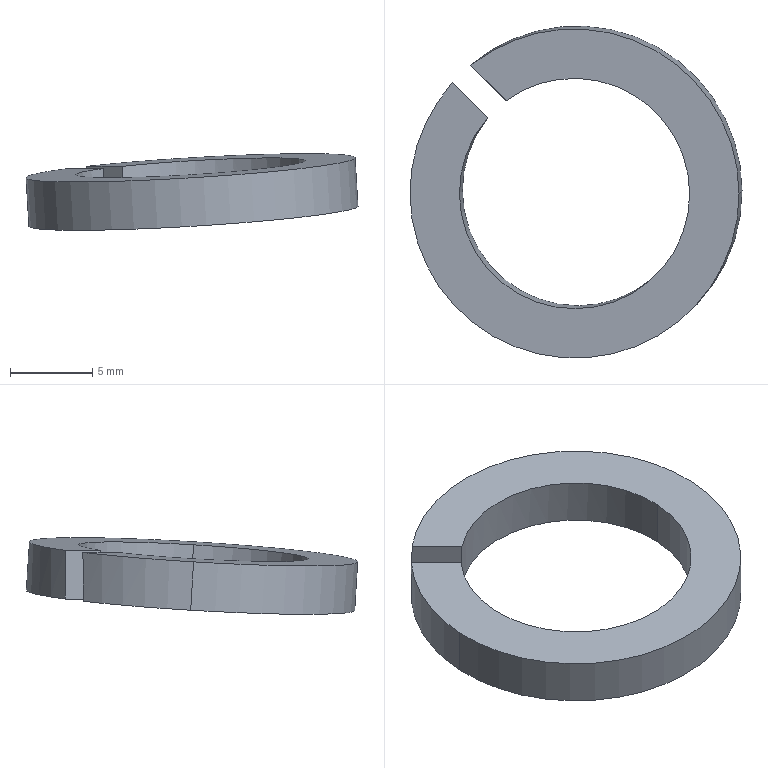Part | SolidWorks | features Boss 1, Cut 1, Extrusion 1, Helix 1, Sweep 1 | 1 solid | 10 faces | box 20.15 x 20.15 x 4.655 mm | volume 458.797 mm3 | cylinder 6 | plane 4 | commonest cylinder face diameters 14 x3 20.008 x3
STEP:
#1=CARTESIAN_POINT('',(-7.602,6.506,0.2121));
#2=VERTEX_POINT('',#1);
#3=CARTESIAN_POINT('',(-10.002,-0.01691,-0.3327));
#4=VERTEX_POINT('',#3);
#5=CARTESIAN_POINT('',(-0.01691,-0.01691,0.2769));
#6=DIRECTION('',(-0.06083,-0.06083,0.9963));
#7=DIRECTION('',(0.9981,0.,0.06094));
#8=AXIS2_PLACEMENT_3D('',#5,#6,#7);
#9=CIRCLE('',#8,10.004);
#10=EDGE_CURVE('',#2,#4,#9,.T.);
#11=ORIENTED_EDGE('',*,*,#10,.T.);
#12=CARTESIAN_POINT('',(-10.181,-0.196,2.601));
#13=VERTEX_POINT('',#12);
#14=CARTESIAN_POINT('',(-10.002,-0.01691,-0.3327));
#15=DIRECTION('',(-0.06083,-0.06083,0.9963));
#16=VECTOR('',#15,1000.);
#17=LINE('',#14,#16);
#18=EDGE_CURVE('',#4,#13,#17,.T.);
#19=ORIENTED_EDGE('',*,*,#18,.T.);
#20=CARTESIAN_POINT('',(-7.613,6.517,3.168));
#21=VERTEX_POINT('',#20);
#22=CARTESIAN_POINT('',(-0.196,-0.196,3.211));
#23=DIRECTION('',(-0.06083,-0.06083,0.9963));
#24=DIRECTION('',(0.9981,0.,0.06094));
#25=AXIS2_PLACEMENT_3D('',#22,#23,#24);
#26=CIRCLE('',#25,10.004);
#27=EDGE_CURVE('',#21,#13,#26,.T.);
#28=ORIENTED_EDGE('',*,*,#27,.F.);
#29=CARTESIAN_POINT('',(-7.602,6.506,0.2121));
#30=CARTESIAN_POINT('',(-7.606,6.51,1.197));
#31=CARTESIAN_POINT('',(-7.61,6.514,2.182));
#32=CARTESIAN_POINT('',(-7.613,6.517,3.168));
#33=(BOUNDED_CURVE()B_SPLINE_CURVE(3,(#29,#30,#31,#32),.UNSPECIFIED.,.F.,.F.)B_SPLINE_CURVE_WITH_KNOTS((4,4),(4.637,4.662),.UNSPECIFIED.)CURVE()GEOMETRIC_REPRESENTATION_ITEM()RATIONAL_B_SPLINE_CURVE((1.,0.9999,0.9999,1.))REPRESENTATION_ITEM(''));
#34=EDGE_CURVE('',#2,#21,#33,.T.);
#35=ORIENTED_EDGE('',*,*,#34,.F.);
#36=EDGE_LOOP('',(#11,#19,#28,#35));
#37=FACE_OUTER_BOUND('',#36,.T.);
#38=CARTESIAN_POINT('',(-0.01691,-0.01691,0.2769));
#39=DIRECTION('',(-0.06083,-0.06083,0.9963));
#40=DIRECTION('',(0.9981,0.,0.06094));
#41=AXIS2_PLACEMENT_3D('',#38,#39,#40);
#42=CYLINDRICAL_SURFACE('',#41,10.004);
#43=ADVANCED_FACE('',(#37),#42,.T.);
#44=ORIENTED_EDGE('',*,*,#18,.F.);
#45=CARTESIAN_POINT('',(9.968,-0.01691,0.8865));
#46=VERTEX_POINT('',#45);
#47=CARTESIAN_POINT('',(-0.01691,-0.01691,0.2769));
#48=DIRECTION('',(-0.06083,-0.06083,0.9963));
#49=DIRECTION('',(0.9981,0.,0.06094));
#50=AXIS2_PLACEMENT_3D('',#47,#48,#49);
#51=CIRCLE('',#50,10.004);
#52=EDGE_CURVE('',#4,#46,#51,.T.);
#53=ORIENTED_EDGE('',*,*,#52,.T.);
#54=CARTESIAN_POINT('',(9.789,-0.196,3.821));
#55=VERTEX_POINT('',#54);
#56=CARTESIAN_POINT('',(9.968,-0.01691,0.8865));
#57=DIRECTION('',(-0.06083,-0.06083,0.9963));
#58=VECTOR('',#57,1000.);
#59=LINE('',#56,#58);
#60=EDGE_CURVE('',#46,#55,#59,.T.);
#61=ORIENTED_EDGE('',*,*,#60,.T.);
#62=CARTESIAN_POINT('',(-0.196,-0.196,3.211));
#63=DIRECTION('',(-0.06083,-0.06083,0.9963));
#64=DIRECTION('',(0.9981,0.,0.06094));
#65=AXIS2_PLACEMENT_3D('',#62,#63,#64);
#66=CIRCLE('',#65,10.004);
#67=EDGE_CURVE('',#13,#55,#66,.T.);
#68=ORIENTED_EDGE('',*,*,#67,.F.);
#69=EDGE_LOOP('',(#44,#53,#61,#68));
#70=FACE_OUTER_BOUND('',#69,.T.);
#71=CARTESIAN_POINT('',(-0.01691,-0.01691,0.2769));
#72=DIRECTION('',(-0.06083,-0.06083,0.9963));
#73=DIRECTION('',(0.9981,0.,0.06094));
#74=AXIS2_PLACEMENT_3D('',#71,#72,#73);
#75=CYLINDRICAL_SURFACE('',#74,10.004);
#76=ADVANCED_FACE('',(#70),#75,.T.);
#77=CARTESIAN_POINT('',(-7.004,-0.01691,-0.1497));
#78=VERTEX_POINT('',#77);
#79=CARTESIAN_POINT('',(6.97,-0.01691,0.7035));
#80=VERTEX_POINT('',#79);
#81=CARTESIAN_POINT('',(-0.01691,-0.01691,0.2769));
#82=DIRECTION('',(-0.06083,-0.06083,0.9963));
#83=DIRECTION('',(0.9981,0.,0.06094));
#84=AXIS2_PLACEMENT_3D('',#81,#82,#83);
#85=CIRCLE('',#84,7.);
#86=EDGE_CURVE('',#78,#80,#85,.T.);
#87=ORIENTED_EDGE('',*,*,#86,.F.);
#88=CARTESIAN_POINT('',(-7.183,-0.196,2.784));
#89=VERTEX_POINT('',#88);
#90=CARTESIAN_POINT('',(-7.004,-0.01691,-0.1497));
#91=DIRECTION('',(-0.06083,-0.06083,0.9963));
#92=VECTOR('',#91,1000.);
#93=LINE('',#90,#92);
#94=EDGE_CURVE('',#78,#89,#93,.T.);
#95=ORIENTED_EDGE('',*,*,#94,.T.);
#96=CARTESIAN_POINT('',(6.791,-0.196,3.638));
#97=VERTEX_POINT('',#96);
#98=CARTESIAN_POINT('',(-0.196,-0.196,3.211));
#99=DIRECTION('',(-0.06083,-0.06083,0.9963));
#100=DIRECTION('',(0.9981,0.,0.06094));
#101=AXIS2_PLACEMENT_3D('',#98,#99,#100);
#102=CIRCLE('',#101,7.);
#103=EDGE_CURVE('',#89,#97,#102,.T.);
#104=ORIENTED_EDGE('',*,*,#103,.T.);
#105=CARTESIAN_POINT('',(6.97,-0.01691,0.7035));
#106=DIRECTION('',(-0.06083,-0.06083,0.9963));
#107=VECTOR('',#106,1000.);
#108=LINE('',#105,#107);
#109=EDGE_CURVE('',#80,#97,#108,.T.);
#110=ORIENTED_EDGE('',*,*,#109,.F.);
#111=EDGE_LOOP('',(#87,#95,#104,#110));
#112=FACE_OUTER_BOUND('',#111,.T.);
#113=CARTESIAN_POINT('',(-0.01691,-0.01691,0.2769));
#114=DIRECTION('',(-0.06083,-0.06083,0.9963));
#115=DIRECTION('',(0.9981,0.,0.06094));
#116=AXIS2_PLACEMENT_3D('',#113,#114,#115);
#117=CYLINDRICAL_SURFACE('',#116,7.);
#118=ADVANCED_FACE('',(#112),#117,.F.);
#119=CARTESIAN_POINT('',(-4.369,5.465,0.3459));
#120=VERTEX_POINT('',#119);
#121=CARTESIAN_POINT('',(-0.01691,-0.01691,0.2769));
#122=DIRECTION('',(-0.06083,-0.06083,0.9963));
#123=DIRECTION('',(0.9981,0.,0.06094));
#124=AXIS2_PLACEMENT_3D('',#121,#122,#123);
#125=CIRCLE('',#124,7.);
#126=EDGE_CURVE('',#80,#120,#125,.T.);
#127=ORIENTED_EDGE('',*,*,#126,.F.);
#128=ORIENTED_EDGE('',*,*,#109,.T.);
#129=CARTESIAN_POINT('',(-4.345,5.441,3.302));
#130=VERTEX_POINT('',#129);
#131=CARTESIAN_POINT('',(-0.196,-0.196,3.211));
#132=DIRECTION('',(-0.06083,-0.06083,0.9963));
#133=DIRECTION('',(0.9981,0.,0.06094));
#134=AXIS2_PLACEMENT_3D('',#131,#132,#133);
#135=CIRCLE('',#134,7.);
#136=EDGE_CURVE('',#97,#130,#135,.T.);
#137=ORIENTED_EDGE('',*,*,#136,.T.);
#138=CARTESIAN_POINT('',(-4.345,5.441,3.302));
#139=CARTESIAN_POINT('',(-4.354,5.45,2.319));
#140=CARTESIAN_POINT('',(-4.362,5.458,1.334));
#141=CARTESIAN_POINT('',(-4.369,5.465,0.3459));
#142=(BOUNDED_CURVE()B_SPLINE_CURVE(3,(#138,#139,#140,#141),.UNSPECIFIED.,.F.,.F.)B_SPLINE_CURVE_WITH_KNOTS((4,4),(1.419,1.456),.UNSPECIFIED.)CURVE()GEOMETRIC_REPRESENTATION_ITEM()RATIONAL_B_SPLINE_CURVE((1.,0.9999,0.9999,1.))REPRESENTATION_ITEM(''));
#143=EDGE_CURVE('',#130,#120,#142,.T.);
#144=ORIENTED_EDGE('',*,*,#143,.T.);
#145=EDGE_LOOP('',(#127,#128,#137,#144));
#146=FACE_OUTER_BOUND('',#145,.T.);
#147=CARTESIAN_POINT('',(-0.01691,-0.01691,0.2769));
#148=DIRECTION('',(-0.06083,-0.06083,0.9963));
#149=DIRECTION('',(0.9981,0.,0.06094));
#150=AXIS2_PLACEMENT_3D('',#147,#148,#149);
#151=CYLINDRICAL_SURFACE('',#150,7.);
#152=ADVANCED_FACE('',(#146),#151,.F.);
#153=CARTESIAN_POINT('',(-5.485,4.389,3.168));
#154=VERTEX_POINT('',#153);
#155=CARTESIAN_POINT('',(-7.605,6.509,3.168));
#156=DIRECTION('',(0.7071,-0.7071,0.));
#157=VECTOR('',#156,1000.);
#158=LINE('',#155,#157);
#159=EDGE_CURVE('',#21,#154,#158,.T.);
#160=ORIENTED_EDGE('',*,*,#159,.F.);
#161=ORIENTED_EDGE('',*,*,#27,.T.);
#162=ORIENTED_EDGE('',*,*,#67,.T.);
#163=CARTESIAN_POINT('',(-6.486,7.582,3.302));
#164=VERTEX_POINT('',#163);
#165=CARTESIAN_POINT('',(-0.196,-0.196,3.211));
#166=DIRECTION('',(-0.06083,-0.06083,0.9963));
#167=DIRECTION('',(0.9981,0.,0.06094));
#168=AXIS2_PLACEMENT_3D('',#165,#166,#167);
#169=CIRCLE('',#168,10.004);
#170=EDGE_CURVE('',#55,#164,#169,.T.);
#171=ORIENTED_EDGE('',*,*,#170,.T.);
#172=CARTESIAN_POINT('',(-6.509,7.605,3.302));
#173=DIRECTION('',(-0.7071,0.7071,0.));
#174=VECTOR('',#173,1000.);
#175=LINE('',#172,#174);
#176=EDGE_CURVE('',#130,#164,#175,.T.);
#177=ORIENTED_EDGE('',*,*,#176,.F.);
#178=ORIENTED_EDGE('',*,*,#136,.F.);
#179=ORIENTED_EDGE('',*,*,#103,.F.);
#180=CARTESIAN_POINT('',(-0.196,-0.196,3.211));
#181=DIRECTION('',(-0.06083,-0.06083,0.9963));
#182=DIRECTION('',(0.9981,0.,0.06094));
#183=AXIS2_PLACEMENT_3D('',#180,#181,#182);
#184=CIRCLE('',#183,7.);
#185=EDGE_CURVE('',#154,#89,#184,.T.);
#186=ORIENTED_EDGE('',*,*,#185,.F.);
#187=EDGE_LOOP('',(#160,#161,#162,#171,#177,#178,#179,#186));
#188=FACE_OUTER_BOUND('',#187,.T.);
#189=CARTESIAN_POINT('',(-7.056,7.057,3.235));
#190=DIRECTION('',(-0.06083,-0.06083,0.9963));
#191=DIRECTION('',(0.9981,0.,0.06094));
#192=AXIS2_PLACEMENT_3D('',#189,#190,#191);
#193=PLANE('',#192);
#194=ADVANCED_FACE('',(#188),#193,.T.);
#195=ORIENTED_EDGE('',*,*,#94,.F.);
#196=CARTESIAN_POINT('',(-5.469,4.373,0.2121));
#197=VERTEX_POINT('',#196);
#198=CARTESIAN_POINT('',(-0.01691,-0.01691,0.2769));
#199=DIRECTION('',(-0.06083,-0.06083,0.9963));
#200=DIRECTION('',(0.9981,0.,0.06094));
#201=AXIS2_PLACEMENT_3D('',#198,#199,#200);
#202=CIRCLE('',#201,7.);
#203=EDGE_CURVE('',#197,#78,#202,.T.);
#204=ORIENTED_EDGE('',*,*,#203,.F.);
#205=CARTESIAN_POINT('',(-5.469,4.373,0.2121));
#206=CARTESIAN_POINT('',(-5.475,4.379,1.196));
#207=CARTESIAN_POINT('',(-5.481,4.385,2.181));
#208=CARTESIAN_POINT('',(-5.485,4.389,3.168));
#209=(BOUNDED_CURVE()B_SPLINE_CURVE(3,(#205,#206,#207,#208),.UNSPECIFIED.,.F.,.F.)B_SPLINE_CURVE_WITH_KNOTS((4,4),(4.604,4.641),.UNSPECIFIED.)CURVE()GEOMETRIC_REPRESENTATION_ITEM()RATIONAL_B_SPLINE_CURVE((1.,0.9999,0.9999,1.))REPRESENTATION_ITEM(''));
#210=EDGE_CURVE('',#197,#154,#209,.T.);
#211=ORIENTED_EDGE('',*,*,#210,.T.);
#212=ORIENTED_EDGE('',*,*,#185,.T.);
#213=EDGE_LOOP('',(#195,#204,#211,#212));
#214=FACE_OUTER_BOUND('',#213,.T.);
#215=CARTESIAN_POINT('',(-0.01691,-0.01691,0.2769));
#216=DIRECTION('',(-0.06083,-0.06083,0.9963));
#217=DIRECTION('',(0.9981,0.,0.06094));
#218=AXIS2_PLACEMENT_3D('',#215,#216,#217);
#219=CYLINDRICAL_SURFACE('',#218,7.);
#220=ADVANCED_FACE('',(#214),#219,.F.);
#221=ORIENTED_EDGE('',*,*,#60,.F.);
#222=CARTESIAN_POINT('',(-6.503,7.599,0.3459));
#223=VERTEX_POINT('',#222);
#224=CARTESIAN_POINT('',(-0.01691,-0.01691,0.2769));
#225=DIRECTION('',(-0.06083,-0.06083,0.9963));
#226=DIRECTION('',(0.9981,0.,0.06094));
#227=AXIS2_PLACEMENT_3D('',#224,#225,#226);
#228=CIRCLE('',#227,10.004);
#229=EDGE_CURVE('',#46,#223,#228,.T.);
#230=ORIENTED_EDGE('',*,*,#229,.T.);
#231=CARTESIAN_POINT('',(-6.486,7.582,3.302));
#232=CARTESIAN_POINT('',(-6.493,7.589,2.318));
#233=CARTESIAN_POINT('',(-6.498,7.594,1.332));
#234=CARTESIAN_POINT('',(-6.503,7.599,0.3459));
#235=(BOUNDED_CURVE()B_SPLINE_CURVE(3,(#231,#232,#233,#234),.UNSPECIFIED.,.F.,.F.)B_SPLINE_CURVE_WITH_KNOTS((4,4),(1.465,1.491),.UNSPECIFIED.)CURVE()GEOMETRIC_REPRESENTATION_ITEM()RATIONAL_B_SPLINE_CURVE((1.,0.9999,0.9999,1.))REPRESENTATION_ITEM(''));
#236=EDGE_CURVE('',#164,#223,#235,.T.);
#237=ORIENTED_EDGE('',*,*,#236,.F.);
#238=ORIENTED_EDGE('',*,*,#170,.F.);
#239=EDGE_LOOP('',(#221,#230,#237,#238));
#240=FACE_OUTER_BOUND('',#239,.T.);
#241=CARTESIAN_POINT('',(-0.01691,-0.01691,0.2769));
#242=DIRECTION('',(-0.06083,-0.06083,0.9963));
#243=DIRECTION('',(0.9981,0.,0.06094));
#244=AXIS2_PLACEMENT_3D('',#241,#242,#243);
#245=CYLINDRICAL_SURFACE('',#244,10.004);
#246=ADVANCED_FACE('',(#240),#245,.T.);
#247=ORIENTED_EDGE('',*,*,#10,.F.);
#248=CARTESIAN_POINT('',(-0.548,-0.548,0.2121));
#249=DIRECTION('',(0.7071,-0.7071,0.));
#250=VECTOR('',#249,1000.);
#251=LINE('',#248,#250);
#252=EDGE_CURVE('',#2,#197,#251,.T.);
#253=ORIENTED_EDGE('',*,*,#252,.T.);
#254=ORIENTED_EDGE('',*,*,#203,.T.);
#255=ORIENTED_EDGE('',*,*,#86,.T.);
#256=ORIENTED_EDGE('',*,*,#126,.T.);
#257=CARTESIAN_POINT('',(0.548,0.548,0.3459));
#258=DIRECTION('',(-0.7071,0.7071,0.));
#259=VECTOR('',#258,1000.);
#260=LINE('',#257,#259);
#261=EDGE_CURVE('',#120,#223,#260,.T.);
#262=ORIENTED_EDGE('',*,*,#261,.T.);
#263=ORIENTED_EDGE('',*,*,#229,.F.);
#264=ORIENTED_EDGE('',*,*,#52,.F.);
#265=EDGE_LOOP('',(#247,#253,#254,#255,#256,#262,#263,#264));
#266=FACE_OUTER_BOUND('',#265,.T.);
#267=CARTESIAN_POINT('',(-0.01691,-0.01691,0.2769));
#268=DIRECTION('',(-0.06083,-0.06083,0.9963));
#269=DIRECTION('',(0.9981,0.,0.06094));
#270=AXIS2_PLACEMENT_3D('',#267,#268,#269);
#271=PLANE('',#270);
#272=ADVANCED_FACE('',(#266),#271,.F.);
#273=ORIENTED_EDGE('',*,*,#176,.T.);
#274=ORIENTED_EDGE('',*,*,#236,.T.);
#275=ORIENTED_EDGE('',*,*,#261,.F.);
#276=ORIENTED_EDGE('',*,*,#143,.F.);
#277=EDGE_LOOP('',(#273,#274,#275,#276));
#278=FACE_OUTER_BOUND('',#277,.T.);
#279=CARTESIAN_POINT('',(-34.703,35.799,-0.5837));
#280=DIRECTION('',(0.7071,0.7071,0.));
#281=DIRECTION('',(-0.7071,0.7071,0.));
#282=AXIS2_PLACEMENT_3D('',#279,#280,#281);
#283=PLANE('',#282);
#284=ADVANCED_FACE('',(#278),#283,.F.);
#285=ORIENTED_EDGE('',*,*,#159,.T.);
#286=ORIENTED_EDGE('',*,*,#210,.F.);
#287=ORIENTED_EDGE('',*,*,#252,.F.);
#288=ORIENTED_EDGE('',*,*,#34,.T.);
#289=EDGE_LOOP('',(#285,#286,#287,#288));
#290=FACE_OUTER_BOUND('',#289,.T.);
#291=CARTESIAN_POINT('',(-0.7972,-0.2988,-0.5837));
#292=DIRECTION('',(-0.7071,-0.7071,0.));
#293=DIRECTION('',(0.7071,-0.7071,0.));
#294=AXIS2_PLACEMENT_3D('',#291,#292,#293);
#295=PLANE('',#294);
#296=ADVANCED_FACE('',(#290),#295,.F.);
#297=CLOSED_SHELL('',(#43,#76,#118,#152,#194,#220,#246,#272,#284,#296));
#298=MANIFOLD_SOLID_BREP('',#297);
#299=CARTESIAN_POINT('',(0.,0.,0.));
#300=DIRECTION('',(0.,0.,1.));
#301=DIRECTION('',(1.,0.,0.));
#302=AXIS2_PLACEMENT_3D('',#299,#300,#301);
#303=(LENGTH_UNIT()NAMED_UNIT(*)SI_UNIT(.MILLI.,.METRE.));
#304=UNCERTAINTY_MEASURE_WITH_UNIT(LENGTH_MEASURE(0.00001),#303,'','');
#305=(NAMED_UNIT(*)PLANE_ANGLE_UNIT()SI_UNIT($,.RADIAN.));
#306=(NAMED_UNIT(*)SI_UNIT($,.STERADIAN.)SOLID_ANGLE_UNIT());
#307=(GEOMETRIC_REPRESENTATION_CONTEXT(3)GLOBAL_UNCERTAINTY_ASSIGNED_CONTEXT((#304))GLOBAL_UNIT_ASSIGNED_CONTEXT((#303,#305,#306))REPRESENTATION_CONTEXT('',''));
#308=ADVANCED_BREP_SHAPE_REPRESENTATION('',(#298,#302),#307);